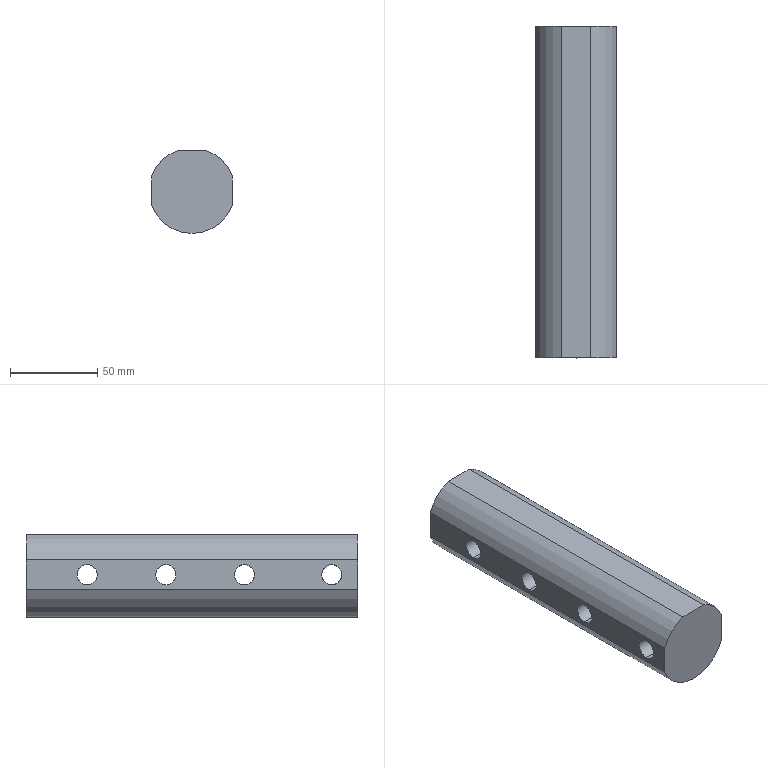Part | SolidWorks | features BaseBody 1 | 1 solid | 28 faces | box 46 x 190 x 47.5 mm | volume 280265 mm3 | cylinder 21 | plane 5 | cone 2 | commonest cylinder face diameters 11.5 x16 49 x3 20 x2